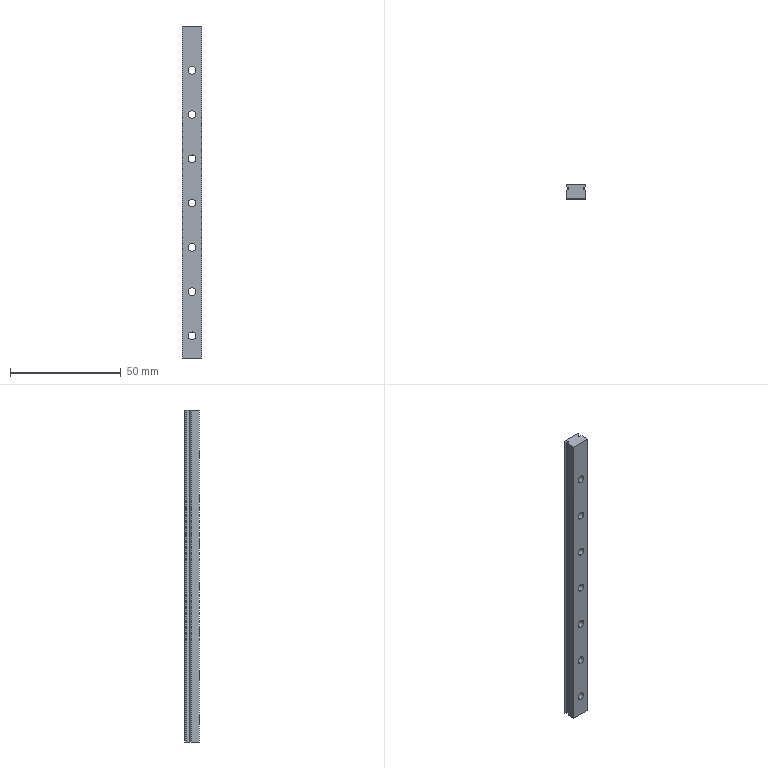Part | SolidWorks | features BaseBody 1 | 1 solid | 70 faces | box 9 x 6.5 x 150 mm | volume 7500 mm3 | cylinder 31 | plane 25 | cone 14 | commonest cylinder face diameters 3.5 x14 5.8 x14 0.8 x3